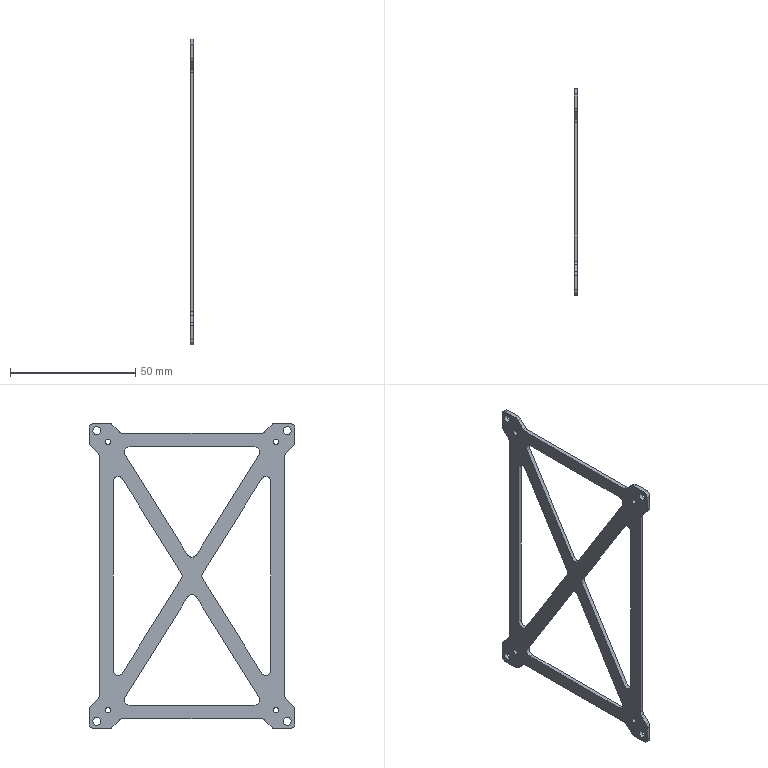Part | SolidWorks | features ICE 2, Extrusion 1, Fillet 1 | 1 solid | 85 faces | box 1.5 x 82 x 122 mm | volume 5369 mm3 | cylinder 51 | plane 34 | commonest cylinder face diameters 4 x35 2.2 x8 3.2 x8